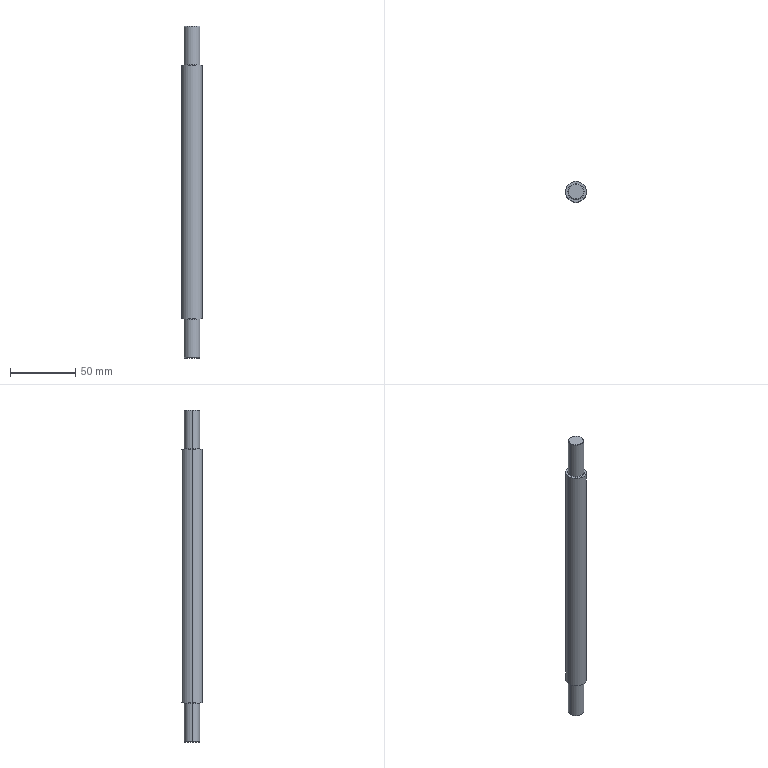Part | STEP file | 0230_002_MTSLW16-255-F30-V12-S30-Q12-BV15 | 1 solid | 18 faces | box 16 x 16 x 255 mm | volume 45988 mm3 | cylinder 6 | cone 4 | torus 4 | plane 4 | commonest cylinder face diameters 12 x4 16 x2
STEP:
#1=CARTESIAN_POINT('',(0.,0.,0.));
#2=DIRECTION('',(0.,0.,1.));
#3=DIRECTION('',(1.,0.,0.));
#4=AXIS2_PLACEMENT_3D('',#1,#2,#3);
#5=CARTESIAN_POINT('',(5.6,0.,30.));
#6=VERTEX_POINT('',#5);
#7=CARTESIAN_POINT('',(-5.6,0.,30.));
#8=VERTEX_POINT('',#7);
#9=CARTESIAN_POINT('',(0.,0.,30.));
#10=DIRECTION('',(0.,0.,1.));
#11=DIRECTION('',(1.,0.,0.));
#12=AXIS2_PLACEMENT_3D('',#9,#10,#11);
#13=CIRCLE('',#12,5.6);
#14=CARTESIAN_POINT('',(0.,0.,29.6));
#15=DIRECTION('',(0.,0.,-1.));
#16=DIRECTION('',(-1.,0.,0.));
#17=AXIS2_PLACEMENT_3D('',#14,#15,#16);
#18=CONICAL_SURFACE('',#17,6.,0.7854);
#19=CARTESIAN_POINT('',(3.142,-0.4));
#20=DIRECTION('',(-1.,0.));
#21=VECTOR('',#20,1.);
#22=LINE('',#19,#21);
#23=(GEOMETRIC_REPRESENTATION_CONTEXT(2)PARAMETRIC_REPRESENTATION_CONTEXT()REPRESENTATION_CONTEXT('',''));
#24=DEFINITIONAL_REPRESENTATION('',(#22),#23);
#25=PCURVE('',#18,#24);
#26=CARTESIAN_POINT('',(6.,0.,30.));
#27=DIRECTION('',(0.,0.,1.));
#28=DIRECTION('',(1.,0.,0.));
#29=AXIS2_PLACEMENT_3D('',#26,#27,#28);
#30=PLANE('',#29);
#31=CARTESIAN_POINT('',(-6.,0.));
#32=DIRECTION('',(1.,0.));
#33=AXIS2_PLACEMENT_2D('',#31,#32);
#34=CIRCLE('',#33,5.6);
#35=(GEOMETRIC_REPRESENTATION_CONTEXT(2)PARAMETRIC_REPRESENTATION_CONTEXT()REPRESENTATION_CONTEXT('',''));
#36=DEFINITIONAL_REPRESENTATION('',(#34),#35);
#37=PCURVE('',#30,#36);
#38=SURFACE_CURVE('',#13,(#25,#37),.PCURVE_S1.);
#39=EDGE_CURVE('',#6,#8,#38,.T.);
#40=ORIENTED_EDGE('',*,*,#39,.F.);
#41=CARTESIAN_POINT('',(6.,0.,29.6));
#42=VERTEX_POINT('',#41);
#43=CARTESIAN_POINT('',(6.,0.,29.6));
#44=DIRECTION('',(0.7071,0.,-0.7071));
#45=VECTOR('',#44,1.);
#46=LINE('',#43,#45);
#47=CARTESIAN_POINT('',(3.142,0.));
#48=DIRECTION('',(0.,1.));
#49=VECTOR('',#48,1.);
#50=LINE('',#47,#49);
#51=(GEOMETRIC_REPRESENTATION_CONTEXT(2)PARAMETRIC_REPRESENTATION_CONTEXT()REPRESENTATION_CONTEXT('',''));
#52=DEFINITIONAL_REPRESENTATION('',(#50),#51);
#53=PCURVE('',#18,#52);
#54=CARTESIAN_POINT('',(0.,0.,29.6));
#55=DIRECTION('',(0.,0.,-1.));
#56=DIRECTION('',(-1.,0.,0.));
#57=AXIS2_PLACEMENT_3D('',#54,#55,#56);
#58=CONICAL_SURFACE('',#57,6.,0.7854);
#59=CARTESIAN_POINT('',(3.142,0.));
#60=DIRECTION('',(0.,1.));
#61=VECTOR('',#60,1.);
#62=LINE('',#59,#61);
#63=(GEOMETRIC_REPRESENTATION_CONTEXT(2)PARAMETRIC_REPRESENTATION_CONTEXT()REPRESENTATION_CONTEXT('',''));
#64=DEFINITIONAL_REPRESENTATION('',(#62),#63);
#65=PCURVE('',#58,#64);
#66=SURFACE_CURVE('',#46,(#53,#65),.PCURVE_S1.);
#67=EDGE_CURVE('',#6,#42,#66,.T.);
#68=ORIENTED_EDGE('',*,*,#67,.T.);
#69=CARTESIAN_POINT('',(-6.,0.,29.6));
#70=VERTEX_POINT('',#69);
#71=CARTESIAN_POINT('',(0.,0.,29.6));
#72=DIRECTION('',(0.,0.,-1.));
#73=DIRECTION('',(1.,0.,0.));
#74=AXIS2_PLACEMENT_3D('',#71,#72,#73);
#75=CIRCLE('',#74,6.);
#76=CARTESIAN_POINT('',(-3.142,0.));
#77=DIRECTION('',(1.,0.));
#78=VECTOR('',#77,1.);
#79=LINE('',#76,#78);
#80=(GEOMETRIC_REPRESENTATION_CONTEXT(2)PARAMETRIC_REPRESENTATION_CONTEXT()REPRESENTATION_CONTEXT('',''));
#81=DEFINITIONAL_REPRESENTATION('',(#79),#80);
#82=PCURVE('',#18,#81);
#83=CARTESIAN_POINT('',(0.,0.,30.));
#84=DIRECTION('',(0.,0.,-1.));
#85=DIRECTION('',(-1.,0.,0.));
#86=AXIS2_PLACEMENT_3D('',#83,#84,#85);
#87=CYLINDRICAL_SURFACE('',#86,6.);
#88=CARTESIAN_POINT('',(-3.142,0.4));
#89=DIRECTION('',(1.,0.));
#90=VECTOR('',#89,1.);
#91=LINE('',#88,#90);
#92=(GEOMETRIC_REPRESENTATION_CONTEXT(2)PARAMETRIC_REPRESENTATION_CONTEXT()REPRESENTATION_CONTEXT('',''));
#93=DEFINITIONAL_REPRESENTATION('',(#91),#92);
#94=PCURVE('',#87,#93);
#95=SURFACE_CURVE('',#75,(#82,#94),.PCURVE_S1.);
#96=EDGE_CURVE('',#70,#42,#95,.T.);
#97=ORIENTED_EDGE('',*,*,#96,.F.);
#98=CARTESIAN_POINT('',(-6.,0.,29.6));
#99=DIRECTION('',(-0.7071,0.,-0.7071));
#100=VECTOR('',#99,1.);
#101=LINE('',#98,#100);
#102=CARTESIAN_POINT('',(0.,0.));
#103=DIRECTION('',(0.,1.));
#104=VECTOR('',#103,1.);
#105=LINE('',#102,#104);
#106=(GEOMETRIC_REPRESENTATION_CONTEXT(2)PARAMETRIC_REPRESENTATION_CONTEXT()REPRESENTATION_CONTEXT('',''));
#107=DEFINITIONAL_REPRESENTATION('',(#105),#106);
#108=PCURVE('',#18,#107);
#109=CARTESIAN_POINT('',(6.283,0.));
#110=DIRECTION('',(0.,1.));
#111=VECTOR('',#110,1.);
#112=LINE('',#109,#111);
#113=(GEOMETRIC_REPRESENTATION_CONTEXT(2)PARAMETRIC_REPRESENTATION_CONTEXT()REPRESENTATION_CONTEXT('',''));
#114=DEFINITIONAL_REPRESENTATION('',(#112),#113);
#115=PCURVE('',#58,#114);
#116=SURFACE_CURVE('',#101,(#108,#115),.PCURVE_S1.);
#117=EDGE_CURVE('',#8,#70,#116,.T.);
#118=ORIENTED_EDGE('',*,*,#117,.F.);
#119=EDGE_LOOP('',(#40,#68,#97,#118));
#120=FACE_BOUND('',#119,.T.);
#121=ADVANCED_FACE('',(#120),#18,.T.);
#122=CARTESIAN_POINT('',(-5.6,0.,-225.));
#123=VERTEX_POINT('',#122);
#124=CARTESIAN_POINT('',(5.6,0.,-225.));
#125=VERTEX_POINT('',#124);
#126=CARTESIAN_POINT('',(0.,0.,-225.));
#127=DIRECTION('',(0.,0.,-1.));
#128=DIRECTION('',(-1.,0.,0.));
#129=AXIS2_PLACEMENT_3D('',#126,#127,#128);
#130=CIRCLE('',#129,5.6);
#131=CARTESIAN_POINT('',(0.,0.,-225.));
#132=DIRECTION('',(0.,0.,1.));
#133=DIRECTION('',(1.,0.,0.));
#134=AXIS2_PLACEMENT_3D('',#131,#132,#133);
#135=CONICAL_SURFACE('',#134,5.6,0.7854);
#136=CARTESIAN_POINT('',(3.142,0.));
#137=DIRECTION('',(-1.,0.));
#138=VECTOR('',#137,1.);
#139=LINE('',#136,#138);
#140=(GEOMETRIC_REPRESENTATION_CONTEXT(2)PARAMETRIC_REPRESENTATION_CONTEXT()REPRESENTATION_CONTEXT('',''));
#141=DEFINITIONAL_REPRESENTATION('',(#139),#140);
#142=PCURVE('',#135,#141);
#143=CARTESIAN_POINT('',(0.,0.,-225.));
#144=DIRECTION('',(0.,0.,-1.));
#145=DIRECTION('',(-1.,0.,0.));
#146=AXIS2_PLACEMENT_3D('',#143,#144,#145);
#147=PLANE('',#146);
#148=CARTESIAN_POINT('',(0.,0.));
#149=DIRECTION('',(1.,0.));
#150=AXIS2_PLACEMENT_2D('',#148,#149);
#151=CIRCLE('',#150,5.6);
#152=(GEOMETRIC_REPRESENTATION_CONTEXT(2)PARAMETRIC_REPRESENTATION_CONTEXT()REPRESENTATION_CONTEXT('',''));
#153=DEFINITIONAL_REPRESENTATION('',(#151),#152);
#154=PCURVE('',#147,#153);
#155=SURFACE_CURVE('',#130,(#142,#154),.PCURVE_S1.);
#156=EDGE_CURVE('',#123,#125,#155,.T.);
#157=ORIENTED_EDGE('',*,*,#156,.F.);
#158=CARTESIAN_POINT('',(-6.,0.,-224.6));
#159=VERTEX_POINT('',#158);
#160=CARTESIAN_POINT('',(-5.6,0.,-225.));
#161=DIRECTION('',(-0.7071,0.,0.7071));
#162=VECTOR('',#161,1.);
#163=LINE('',#160,#162);
#164=CARTESIAN_POINT('',(3.142,0.));
#165=DIRECTION('',(0.,1.));
#166=VECTOR('',#165,1.);
#167=LINE('',#164,#166);
#168=(GEOMETRIC_REPRESENTATION_CONTEXT(2)PARAMETRIC_REPRESENTATION_CONTEXT()REPRESENTATION_CONTEXT('',''));
#169=DEFINITIONAL_REPRESENTATION('',(#167),#168);
#170=PCURVE('',#135,#169);
#171=CARTESIAN_POINT('',(0.,0.,-225.));
#172=DIRECTION('',(0.,0.,1.));
#173=DIRECTION('',(1.,0.,0.));
#174=AXIS2_PLACEMENT_3D('',#171,#172,#173);
#175=CONICAL_SURFACE('',#174,5.6,0.7854);
#176=CARTESIAN_POINT('',(3.142,0.));
#177=DIRECTION('',(0.,1.));
#178=VECTOR('',#177,1.);
#179=LINE('',#176,#178);
#180=(GEOMETRIC_REPRESENTATION_CONTEXT(2)PARAMETRIC_REPRESENTATION_CONTEXT()REPRESENTATION_CONTEXT('',''));
#181=DEFINITIONAL_REPRESENTATION('',(#179),#180);
#182=PCURVE('',#175,#181);
#183=SURFACE_CURVE('',#163,(#170,#182),.PCURVE_S1.);
#184=EDGE_CURVE('',#123,#159,#183,.T.);
#185=ORIENTED_EDGE('',*,*,#184,.T.);
#186=CARTESIAN_POINT('',(6.,0.,-224.6));
#187=VERTEX_POINT('',#186);
#188=CARTESIAN_POINT('',(0.,0.,-224.6));
#189=DIRECTION('',(0.,0.,1.));
#190=DIRECTION('',(-1.,0.,0.));
#191=AXIS2_PLACEMENT_3D('',#188,#189,#190);
#192=CIRCLE('',#191,6.);
#193=CARTESIAN_POINT('',(-3.142,0.4));
#194=DIRECTION('',(1.,0.));
#195=VECTOR('',#194,1.);
#196=LINE('',#193,#195);
#197=(GEOMETRIC_REPRESENTATION_CONTEXT(2)PARAMETRIC_REPRESENTATION_CONTEXT()REPRESENTATION_CONTEXT('',''));
#198=DEFINITIONAL_REPRESENTATION('',(#196),#197);
#199=PCURVE('',#135,#198);
#200=CARTESIAN_POINT('',(0.,0.,30.));
#201=DIRECTION('',(0.,0.,-1.));
#202=DIRECTION('',(-1.,0.,0.));
#203=AXIS2_PLACEMENT_3D('',#200,#201,#202);
#204=CYLINDRICAL_SURFACE('',#203,6.);
#205=CARTESIAN_POINT('',(6.283,254.6));
#206=DIRECTION('',(-1.,0.));
#207=VECTOR('',#206,1.);
#208=LINE('',#205,#207);
#209=(GEOMETRIC_REPRESENTATION_CONTEXT(2)PARAMETRIC_REPRESENTATION_CONTEXT()REPRESENTATION_CONTEXT('',''));
#210=DEFINITIONAL_REPRESENTATION('',(#208),#209);
#211=PCURVE('',#204,#210);
#212=SURFACE_CURVE('',#192,(#199,#211),.PCURVE_S1.);
#213=EDGE_CURVE('',#187,#159,#212,.T.);
#214=ORIENTED_EDGE('',*,*,#213,.F.);
#215=CARTESIAN_POINT('',(5.6,0.,-225.));
#216=DIRECTION('',(0.7071,0.,0.7071));
#217=VECTOR('',#216,1.);
#218=LINE('',#215,#217);
#219=CARTESIAN_POINT('',(0.,0.));
#220=DIRECTION('',(0.,1.));
#221=VECTOR('',#220,1.);
#222=LINE('',#219,#221);
#223=(GEOMETRIC_REPRESENTATION_CONTEXT(2)PARAMETRIC_REPRESENTATION_CONTEXT()REPRESENTATION_CONTEXT('',''));
#224=DEFINITIONAL_REPRESENTATION('',(#222),#223);
#225=PCURVE('',#135,#224);
#226=CARTESIAN_POINT('',(6.283,0.));
#227=DIRECTION('',(0.,1.));
#228=VECTOR('',#227,1.);
#229=LINE('',#226,#228);
#230=(GEOMETRIC_REPRESENTATION_CONTEXT(2)PARAMETRIC_REPRESENTATION_CONTEXT()REPRESENTATION_CONTEXT('',''));
#231=DEFINITIONAL_REPRESENTATION('',(#229),#230);
#232=PCURVE('',#175,#231);
#233=SURFACE_CURVE('',#218,(#225,#232),.PCURVE_S1.);
#234=EDGE_CURVE('',#125,#187,#233,.T.);
#235=ORIENTED_EDGE('',*,*,#234,.F.);
#236=EDGE_LOOP('',(#157,#185,#214,#235));
#237=FACE_BOUND('',#236,.T.);
#238=ADVANCED_FACE('',(#237),#135,.T.);
#239=CARTESIAN_POINT('',(6.,0.,0.3));
#240=VERTEX_POINT('',#239);
#241=CARTESIAN_POINT('',(6.3,0.,0.));
#242=VERTEX_POINT('',#241);
#243=CARTESIAN_POINT('',(6.3,0.,0.3));
#244=DIRECTION('',(0.,-1.,0.));
#245=DIRECTION('',(0.,0.,-1.));
#246=AXIS2_PLACEMENT_3D('',#243,#244,#245);
#247=CIRCLE('',#246,0.3);
#248=CARTESIAN_POINT('',(0.,0.,0.3));
#249=DIRECTION('',(0.,0.,1.));
#250=DIRECTION('',(1.,0.,0.));
#251=AXIS2_PLACEMENT_3D('',#248,#249,#250);
#252=TOROIDAL_SURFACE('',#251,6.3,0.3);
#253=CARTESIAN_POINT('',(6.283,-1.571));
#254=DIRECTION('',(0.,1.));
#255=VECTOR('',#254,1.);
#256=LINE('',#253,#255);
#257=(GEOMETRIC_REPRESENTATION_CONTEXT(2)PARAMETRIC_REPRESENTATION_CONTEXT()REPRESENTATION_CONTEXT('',''));
#258=DEFINITIONAL_REPRESENTATION('',(#256),#257);
#259=PCURVE('',#252,#258);
#260=CARTESIAN_POINT('',(0.,0.,0.3));
#261=DIRECTION('',(0.,0.,1.));
#262=DIRECTION('',(1.,0.,0.));
#263=AXIS2_PLACEMENT_3D('',#260,#261,#262);
#264=TOROIDAL_SURFACE('',#263,6.3,0.3);
#265=CARTESIAN_POINT('',(0.,-1.571));
#266=DIRECTION('',(0.,1.));
#267=VECTOR('',#266,1.);
#268=LINE('',#265,#267);
#269=(GEOMETRIC_REPRESENTATION_CONTEXT(2)PARAMETRIC_REPRESENTATION_CONTEXT()REPRESENTATION_CONTEXT('',''));
#270=DEFINITIONAL_REPRESENTATION('',(#268),#269);
#271=PCURVE('',#264,#270);
#272=SURFACE_CURVE('',#247,(#259,#271),.PCURVE_S1.);
#273=EDGE_CURVE('',#240,#242,#272,.T.);
#274=ORIENTED_EDGE('',*,*,#273,.T.);
#275=CARTESIAN_POINT('',(-6.3,0.,0.));
#276=VERTEX_POINT('',#275);
#277=CARTESIAN_POINT('',(0.,0.,0.));
#278=DIRECTION('',(0.,0.,-1.));
#279=DIRECTION('',(1.,0.,0.));
#280=AXIS2_PLACEMENT_3D('',#277,#278,#279);
#281=CIRCLE('',#280,6.3);
#282=CARTESIAN_POINT('',(6.283,4.712));
#283=DIRECTION('',(-1.,0.));
#284=VECTOR('',#283,1.);
#285=LINE('',#282,#284);
#286=(GEOMETRIC_REPRESENTATION_CONTEXT(2)PARAMETRIC_REPRESENTATION_CONTEXT()REPRESENTATION_CONTEXT('',''));
#287=DEFINITIONAL_REPRESENTATION('',(#285),#286);
#288=PCURVE('',#252,#287);
#289=CARTESIAN_POINT('',(8.,0.,0.));
#290=DIRECTION('',(0.,0.,1.));
#291=DIRECTION('',(1.,0.,0.));
#292=AXIS2_PLACEMENT_3D('',#289,#290,#291);
#293=PLANE('',#292);
#294=CARTESIAN_POINT('',(-1.7,0.));
#295=CARTESIAN_POINT('',(-1.7,-10.912));
#296=CARTESIAN_POINT('',(-11.15,-5.456));
#297=CARTESIAN_POINT('',(-20.6,0.));
#298=CARTESIAN_POINT('',(-11.15,5.456));
#299=CARTESIAN_POINT('',(-1.7,10.912));
#300=CARTESIAN_POINT('',(-1.7,0.));
#301=(BOUNDED_CURVE()B_SPLINE_CURVE(2,(#294,#295,#296,#297,#298,#299,#300),.UNSPECIFIED.,.T.,.F.)B_SPLINE_CURVE_WITH_KNOTS((1,2,2,2,2,1),(-2.094,0.,2.094,4.189,6.283,8.378),.UNSPECIFIED.)CURVE()GEOMETRIC_REPRESENTATION_ITEM()RATIONAL_B_SPLINE_CURVE((1.,0.5,1.,0.5,1.,0.5,1.))REPRESENTATION_ITEM(''));
#302=(GEOMETRIC_REPRESENTATION_CONTEXT(2)PARAMETRIC_REPRESENTATION_CONTEXT()REPRESENTATION_CONTEXT('',''));
#303=DEFINITIONAL_REPRESENTATION('',(#301),#302);
#304=PCURVE('',#293,#303);
#305=SURFACE_CURVE('',#281,(#288,#304),.PCURVE_S1.);
#306=EDGE_CURVE('',#242,#276,#305,.T.);
#307=ORIENTED_EDGE('',*,*,#306,.T.);
#308=CARTESIAN_POINT('',(-6.,0.,0.3));
#309=VERTEX_POINT('',#308);
#310=CARTESIAN_POINT('',(-6.3,0.,0.3));
#311=DIRECTION('',(0.,1.,0.));
#312=DIRECTION('',(-1.,0.,0.));
#313=AXIS2_PLACEMENT_3D('',#310,#311,#312);
#314=CIRCLE('',#313,0.3);
#315=CARTESIAN_POINT('',(3.142,0.));
#316=DIRECTION('',(0.,1.));
#317=VECTOR('',#316,1.);
#318=LINE('',#315,#317);
#319=(GEOMETRIC_REPRESENTATION_CONTEXT(2)PARAMETRIC_REPRESENTATION_CONTEXT()REPRESENTATION_CONTEXT('',''));
#320=DEFINITIONAL_REPRESENTATION('',(#318),#319);
#321=PCURVE('',#252,#320);
#322=CARTESIAN_POINT('',(3.142,0.));
#323=DIRECTION('',(0.,1.));
#324=VECTOR('',#323,1.);
#325=LINE('',#322,#324);
#326=(GEOMETRIC_REPRESENTATION_CONTEXT(2)PARAMETRIC_REPRESENTATION_CONTEXT()REPRESENTATION_CONTEXT('',''));
#327=DEFINITIONAL_REPRESENTATION('',(#325),#326);
#328=PCURVE('',#264,#327);
#329=SURFACE_CURVE('',#314,(#321,#328),.PCURVE_S1.);
#330=EDGE_CURVE('',#309,#276,#329,.T.);
#331=ORIENTED_EDGE('',*,*,#330,.F.);
#332=CARTESIAN_POINT('',(0.,0.,0.3));
#333=DIRECTION('',(0.,0.,1.));
#334=DIRECTION('',(1.,0.,0.));
#335=AXIS2_PLACEMENT_3D('',#332,#333,#334);
#336=CIRCLE('',#335,6.);
#337=CARTESIAN_POINT('',(0.,3.142));
#338=DIRECTION('',(1.,0.));
#339=VECTOR('',#338,1.);
#340=LINE('',#337,#339);
#341=(GEOMETRIC_REPRESENTATION_CONTEXT(2)PARAMETRIC_REPRESENTATION_CONTEXT()REPRESENTATION_CONTEXT('',''));
#342=DEFINITIONAL_REPRESENTATION('',(#340),#341);
#343=PCURVE('',#252,#342);
#344=CARTESIAN_POINT('',(0.,0.,30.));
#345=DIRECTION('',(0.,0.,-1.));
#346=DIRECTION('',(-1.,0.,0.));
#347=AXIS2_PLACEMENT_3D('',#344,#345,#346);
#348=CYLINDRICAL_SURFACE('',#347,6.);
#349=CARTESIAN_POINT('',(9.425,29.7));
#350=DIRECTION('',(-1.,0.));
#351=VECTOR('',#350,1.);
#352=LINE('',#349,#351);
#353=(GEOMETRIC_REPRESENTATION_CONTEXT(2)PARAMETRIC_REPRESENTATION_CONTEXT()REPRESENTATION_CONTEXT('',''));
#354=DEFINITIONAL_REPRESENTATION('',(#352),#353);
#355=PCURVE('',#348,#354);
#356=SURFACE_CURVE('',#336,(#343,#355),.PCURVE_S1.);
#357=EDGE_CURVE('',#309,#240,#356,.T.);
#358=ORIENTED_EDGE('',*,*,#357,.T.);
#359=EDGE_LOOP('',(#274,#307,#331,#358));
#360=FACE_BOUND('',#359,.F.);
#361=ADVANCED_FACE('',(#360),#252,.F.);
#362=CARTESIAN_POINT('',(-6.,0.,-195.3));
#363=VERTEX_POINT('',#362);
#364=CARTESIAN_POINT('',(-6.3,0.,-195.));
#365=VERTEX_POINT('',#364);
#366=CARTESIAN_POINT('',(-6.3,0.,-195.3));
#367=DIRECTION('',(0.,-1.,0.));
#368=DIRECTION('',(0.,0.,-1.));
#369=AXIS2_PLACEMENT_3D('',#366,#367,#368);
#370=CIRCLE('',#369,0.3);
#371=CARTESIAN_POINT('',(0.,0.,-195.3));
#372=DIRECTION('',(0.,0.,-1.));
#373=DIRECTION('',(-1.,0.,0.));
#374=AXIS2_PLACEMENT_3D('',#371,#372,#373);
#375=TOROIDAL_SURFACE('',#374,6.3,0.3);
#376=CARTESIAN_POINT('',(6.283,1.571));
#377=DIRECTION('',(0.,1.));
#378=VECTOR('',#377,1.);
#379=LINE('',#376,#378);
#380=(GEOMETRIC_REPRESENTATION_CONTEXT(2)PARAMETRIC_REPRESENTATION_CONTEXT()REPRESENTATION_CONTEXT('',''));
#381=DEFINITIONAL_REPRESENTATION('',(#379),#380);
#382=PCURVE('',#375,#381);
#383=CARTESIAN_POINT('',(0.,0.,-195.3));
#384=DIRECTION('',(0.,0.,-1.));
#385=DIRECTION('',(-1.,0.,0.));
#386=AXIS2_PLACEMENT_3D('',#383,#384,#385);
#387=TOROIDAL_SURFACE('',#386,6.3,0.3);
#388=CARTESIAN_POINT('',(0.,1.571));
#389=DIRECTION('',(0.,1.));
#390=VECTOR('',#389,1.);
#391=LINE('',#388,#390);
#392=(GEOMETRIC_REPRESENTATION_CONTEXT(2)PARAMETRIC_REPRESENTATION_CONTEXT()REPRESENTATION_CONTEXT('',''));
#393=DEFINITIONAL_REPRESENTATION('',(#391),#392);
#394=PCURVE('',#387,#393);
#395=SURFACE_CURVE('',#370,(#382,#394),.PCURVE_S1.);
#396=EDGE_CURVE('',#363,#365,#395,.T.);
#397=ORIENTED_EDGE('',*,*,#396,.T.);
#398=CARTESIAN_POINT('',(6.3,0.,-195.));
#399=VERTEX_POINT('',#398);
#400=CARTESIAN_POINT('',(0.,0.,-195.));
#401=DIRECTION('',(0.,0.,1.));
#402=DIRECTION('',(-1.,0.,0.));
#403=AXIS2_PLACEMENT_3D('',#400,#401,#402);
#404=CIRCLE('',#403,6.3);
#405=CARTESIAN_POINT('',(6.283,4.712));
#406=DIRECTION('',(-1.,0.));
#407=VECTOR('',#406,1.);
#408=LINE('',#405,#407);
#409=(GEOMETRIC_REPRESENTATION_CONTEXT(2)PARAMETRIC_REPRESENTATION_CONTEXT()REPRESENTATION_CONTEXT('',''));
#410=DEFINITIONAL_REPRESENTATION('',(#408),#409);
#411=PCURVE('',#375,#410);
#412=CARTESIAN_POINT('',(6.,0.,-195.));
#413=DIRECTION('',(0.,0.,-1.));
#414=DIRECTION('',(-1.,0.,0.));
#415=AXIS2_PLACEMENT_3D('',#412,#413,#414);
#416=PLANE('',#415);
#417=CARTESIAN_POINT('',(12.3,0.));
#418=CARTESIAN_POINT('',(12.3,-10.912));
#419=CARTESIAN_POINT('',(2.85,-5.456));
#420=CARTESIAN_POINT('',(-6.6,0.));
#421=CARTESIAN_POINT('',(2.85,5.456));
#422=CARTESIAN_POINT('',(12.3,10.912));
#423=CARTESIAN_POINT('',(12.3,0.));
#424=(BOUNDED_CURVE()B_SPLINE_CURVE(2,(#417,#418,#419,#420,#421,#422,#423),.UNSPECIFIED.,.T.,.F.)B_SPLINE_CURVE_WITH_KNOTS((1,2,2,2,2,1),(-2.094,0.,2.094,4.189,6.283,8.378),.UNSPECIFIED.)CURVE()GEOMETRIC_REPRESENTATION_ITEM()RATIONAL_B_SPLINE_CURVE((1.,0.5,1.,0.5,1.,0.5,1.))REPRESENTATION_ITEM(''));
#425=(GEOMETRIC_REPRESENTATION_CONTEXT(2)PARAMETRIC_REPRESENTATION_CONTEXT()REPRESENTATION_CONTEXT('',''));
#426=DEFINITIONAL_REPRESENTATION('',(#424),#425);
#427=PCURVE('',#416,#426);
#428=SURFACE_CURVE('',#404,(#411,#427),.PCURVE_S1.);
#429=EDGE_CURVE('',#365,#399,#428,.T.);
#430=ORIENTED_EDGE('',*,*,#429,.T.);
#431=CARTESIAN_POINT('',(6.,0.,-195.3));
#432=VERTEX_POINT('',#431);
#433=CARTESIAN_POINT('',(6.3,0.,-195.3));
#434=DIRECTION('',(0.,1.,0.));
#435=DIRECTION('',(-1.,0.,0.));
#436=AXIS2_PLACEMENT_3D('',#433,#434,#435);
#437=CIRCLE('',#436,0.3);
#438=CARTESIAN_POINT('',(3.142,3.142));
#439=DIRECTION('',(0.,1.));
#440=VECTOR('',#439,1.);
#441=LINE('',#438,#440);
#442=(GEOMETRIC_REPRESENTATION_CONTEXT(2)PARAMETRIC_REPRESENTATION_CONTEXT()REPRESENTATION_CONTEXT('',''));
#443=DEFINITIONAL_REPRESENTATION('',(#441),#442);
#444=PCURVE('',#375,#443);
#445=CARTESIAN_POINT('',(3.142,3.142));
#446=DIRECTION('',(0.,1.));
#447=VECTOR('',#446,1.);
#448=LINE('',#445,#447);
#449=(GEOMETRIC_REPRESENTATION_CONTEXT(2)PARAMETRIC_REPRESENTATION_CONTEXT()REPRESENTATION_CONTEXT('',''));
#450=DEFINITIONAL_REPRESENTATION('',(#448),#449);
#451=PCURVE('',#387,#450);
#452=SURFACE_CURVE('',#437,(#444,#451),.PCURVE_S1.);
#453=EDGE_CURVE('',#432,#399,#452,.T.);
#454=ORIENTED_EDGE('',*,*,#453,.F.);
#455=CARTESIAN_POINT('',(0.,0.,-195.3));
#456=DIRECTION('',(0.,0.,-1.));
#457=DIRECTION('',(-1.,0.,0.));
#458=AXIS2_PLACEMENT_3D('',#455,#456,#457);
#459=CIRCLE('',#458,6.);
#460=CARTESIAN_POINT('',(0.,3.142));
#461=DIRECTION('',(1.,0.));
#462=VECTOR('',#461,1.);
#463=LINE('',#460,#462);
#464=(GEOMETRIC_REPRESENTATION_CONTEXT(2)PARAMETRIC_REPRESENTATION_CONTEXT()REPRESENTATION_CONTEXT('',''));
#465=DEFINITIONAL_REPRESENTATION('',(#463),#464);
#466=PCURVE('',#375,#465);
#467=CARTESIAN_POINT('',(0.,0.,30.));
#468=DIRECTION('',(0.,0.,-1.));
#469=DIRECTION('',(-1.,0.,0.));
#470=AXIS2_PLACEMENT_3D('',#467,#468,#469);
#471=CYLINDRICAL_SURFACE('',#470,6.);
#472=CARTESIAN_POINT('',(0.,225.3));
#473=DIRECTION('',(1.,0.));
#474=VECTOR('',#473,1.);
#475=LINE('',#472,#474);
#476=(GEOMETRIC_REPRESENTATION_CONTEXT(2)PARAMETRIC_REPRESENTATION_CONTEXT()REPRESENTATION_CONTEXT('',''));
#477=DEFINITIONAL_REPRESENTATION('',(#475),#476);
#478=PCURVE('',#471,#477);
#479=SURFACE_CURVE('',#459,(#466,#478),.PCURVE_S1.);
#480=EDGE_CURVE('',#432,#363,#479,.T.);
#481=ORIENTED_EDGE('',*,*,#480,.T.);
#482=EDGE_LOOP('',(#397,#430,#454,#481));
#483=FACE_BOUND('',#482,.F.);
#484=ADVANCED_FACE('',(#483),#375,.F.);
#485=CARTESIAN_POINT('',(-8.,0.,0.));
#486=VERTEX_POINT('',#485);
#487=CARTESIAN_POINT('',(8.,0.,0.));
#488=VERTEX_POINT('',#487);
#489=CARTESIAN_POINT('',(0.,0.,0.));
#490=DIRECTION('',(0.,0.,-1.));
#491=DIRECTION('',(-1.,0.,0.));
#492=AXIS2_PLACEMENT_3D('',#489,#490,#491);
#493=CIRCLE('',#492,8.);
#494=CARTESIAN_POINT('',(0.,0.,30.));
#495=DIRECTION('',(0.,0.,-1.));
#496=DIRECTION('',(-1.,0.,0.));
#497=AXIS2_PLACEMENT_3D('',#494,#495,#496);
#498=CYLINDRICAL_SURFACE('',#497,8.);
#499=CARTESIAN_POINT('',(0.,30.));
#500=DIRECTION('',(1.,0.));
#501=VECTOR('',#500,1.);
#502=LINE('',#499,#501);
#503=(GEOMETRIC_REPRESENTATION_CONTEXT(2)PARAMETRIC_REPRESENTATION_CONTEXT()REPRESENTATION_CONTEXT('',''));
#504=DEFINITIONAL_REPRESENTATION('',(#502),#503);
#505=PCURVE('',#498,#504);
#506=CARTESIAN_POINT('',(-16.,0.));
#507=CARTESIAN_POINT('',(-16.,13.856));
#508=CARTESIAN_POINT('',(-4.,6.928));
#509=CARTESIAN_POINT('',(8.,0.));
#510=CARTESIAN_POINT('',(-4.,-6.928));
#511=CARTESIAN_POINT('',(-16.,-13.856));
#512=CARTESIAN_POINT('',(-16.,0.));
#513=(BOUNDED_CURVE()B_SPLINE_CURVE(2,(#506,#507,#508,#509,#510,#511,#512),.UNSPECIFIED.,.T.,.F.)B_SPLINE_CURVE_WITH_KNOTS((1,2,2,2,2,1),(-2.094,0.,2.094,4.189,6.283,8.378),.UNSPECIFIED.)CURVE()GEOMETRIC_REPRESENTATION_ITEM()RATIONAL_B_SPLINE_CURVE((1.,0.5,1.,0.5,1.,0.5,1.))REPRESENTATION_ITEM(''));
#514=(GEOMETRIC_REPRESENTATION_CONTEXT(2)PARAMETRIC_REPRESENTATION_CONTEXT()REPRESENTATION_CONTEXT('',''));
#515=DEFINITIONAL_REPRESENTATION('',(#513),#514);
#516=PCURVE('',#293,#515);
#517=SURFACE_CURVE('',#493,(#505,#516),.PCURVE_S1.);
#518=EDGE_CURVE('',#486,#488,#517,.T.);
#519=ORIENTED_EDGE('',*,*,#518,.T.);
#520=CARTESIAN_POINT('',(8.,0.,-195.));
#521=VERTEX_POINT('',#520);
#522=CARTESIAN_POINT('',(8.,0.,30.));
#523=DIRECTION('',(0.,0.,-1.));
#524=VECTOR('',#523,1.);
#525=LINE('',#522,#524);
#526=CARTESIAN_POINT('',(3.142,0.));
#527=DIRECTION('',(0.,1.));
#528=VECTOR('',#527,1.);
#529=LINE('',#526,#528);
#530=(GEOMETRIC_REPRESENTATION_CONTEXT(2)PARAMETRIC_REPRESENTATION_CONTEXT()REPRESENTATION_CONTEXT('',''));
#531=DEFINITIONAL_REPRESENTATION('',(#529),#530);
#532=PCURVE('',#498,#531);
#533=CARTESIAN_POINT('',(0.,0.,30.));
#534=DIRECTION('',(0.,0.,-1.));
#535=DIRECTION('',(-1.,0.,0.));
#536=AXIS2_PLACEMENT_3D('',#533,#534,#535);
#537=CYLINDRICAL_SURFACE('',#536,8.);
#538=CARTESIAN_POINT('',(3.142,0.));
#539=DIRECTION('',(0.,1.));
#540=VECTOR('',#539,1.);
#541=LINE('',#538,#540);
#542=(GEOMETRIC_REPRESENTATION_CONTEXT(2)PARAMETRIC_REPRESENTATION_CONTEXT()REPRESENTATION_CONTEXT('',''));
#543=DEFINITIONAL_REPRESENTATION('',(#541),#542);
#544=PCURVE('',#537,#543);
#545=SURFACE_CURVE('',#525,(#532,#544),.PCURVE_S1.);
#546=EDGE_CURVE('',#488,#521,#545,.T.);
#547=ORIENTED_EDGE('',*,*,#546,.T.);
#548=CARTESIAN_POINT('',(-8.,0.,-195.));
#549=VERTEX_POINT('',#548);
#550=CARTESIAN_POINT('',(0.,0.,-195.));
#551=DIRECTION('',(0.,0.,-1.));
#552=DIRECTION('',(-1.,0.,0.));
#553=AXIS2_PLACEMENT_3D('',#550,#551,#552);
#554=CIRCLE('',#553,8.);
#555=CARTESIAN_POINT('',(0.,225.));
#556=DIRECTION('',(1.,0.));
#557=VECTOR('',#556,1.);
#558=LINE('',#555,#557);
#559=(GEOMETRIC_REPRESENTATION_CONTEXT(2)PARAMETRIC_REPRESENTATION_CONTEXT()REPRESENTATION_CONTEXT('',''));
#560=DEFINITIONAL_REPRESENTATION('',(#558),#559);
#561=PCURVE('',#498,#560);
#562=CARTESIAN_POINT('',(6.,0.));
#563=DIRECTION('',(1.,0.));
#564=AXIS2_PLACEMENT_2D('',#562,#563);
#565=CIRCLE('',#564,8.);
#566=(GEOMETRIC_REPRESENTATION_CONTEXT(2)PARAMETRIC_REPRESENTATION_CONTEXT()REPRESENTATION_CONTEXT('',''));
#567=DEFINITIONAL_REPRESENTATION('',(#565),#566);
#568=PCURVE('',#416,#567);
#569=SURFACE_CURVE('',#554,(#561,#568),.PCURVE_S1.);
#570=EDGE_CURVE('',#549,#521,#569,.T.);
#571=ORIENTED_EDGE('',*,*,#570,.F.);
#572=CARTESIAN_POINT('',(-8.,0.,30.));
#573=DIRECTION('',(0.,0.,-1.));
#574=VECTOR('',#573,1.);
#575=LINE('',#572,#574);
#576=CARTESIAN_POINT('',(0.,0.));
#577=DIRECTION('',(0.,1.));
#578=VECTOR('',#577,1.);
#579=LINE('',#576,#578);
#580=(GEOMETRIC_REPRESENTATION_CONTEXT(2)PARAMETRIC_REPRESENTATION_CONTEXT()REPRESENTATION_CONTEXT('',''));
#581=DEFINITIONAL_REPRESENTATION('',(#579),#580);
#582=PCURVE('',#498,#581);
#583=CARTESIAN_POINT('',(6.283,0.));
#584=DIRECTION('',(0.,1.));
#585=VECTOR('',#584,1.);
#586=LINE('',#583,#585);
#587=(GEOMETRIC_REPRESENTATION_CONTEXT(2)PARAMETRIC_REPRESENTATION_CONTEXT()REPRESENTATION_CONTEXT('',''));
#588=DEFINITIONAL_REPRESENTATION('',(#586),#587);
#589=PCURVE('',#537,#588);
#590=SURFACE_CURVE('',#575,(#582,#589),.PCURVE_S1.);
#591=EDGE_CURVE('',#486,#549,#590,.T.);
#592=ORIENTED_EDGE('',*,*,#591,.F.);
#593=EDGE_LOOP('',(#519,#547,#571,#592));
#594=FACE_BOUND('',#593,.T.);
#595=ADVANCED_FACE('',(#594),#498,.T.);
#596=CARTESIAN_POINT('',(0.,0.,-195.3));
#597=DIRECTION('',(0.,0.,-1.));
#598=DIRECTION('',(-1.,0.,0.));
#599=AXIS2_PLACEMENT_3D('',#596,#597,#598);
#600=CIRCLE('',#599,6.);
#601=CARTESIAN_POINT('',(0.,225.3));
#602=DIRECTION('',(1.,0.));
#603=VECTOR('',#602,1.);
#604=LINE('',#601,#603);
#605=(GEOMETRIC_REPRESENTATION_CONTEXT(2)PARAMETRIC_REPRESENTATION_CONTEXT()REPRESENTATION_CONTEXT('',''));
#606=DEFINITIONAL_REPRESENTATION('',(#604),#605);
#607=PCURVE('',#204,#606);
#608=CARTESIAN_POINT('',(0.,3.142));
#609=DIRECTION('',(1.,0.));
#610=VECTOR('',#609,1.);
#611=LINE('',#608,#610);
#612=(GEOMETRIC_REPRESENTATION_CONTEXT(2)PARAMETRIC_REPRESENTATION_CONTEXT()REPRESENTATION_CONTEXT('',''));
#613=DEFINITIONAL_REPRESENTATION('',(#611),#612);
#614=PCURVE('',#387,#613);
#615=SURFACE_CURVE('',#600,(#607,#614),.PCURVE_S1.);
#616=EDGE_CURVE('',#363,#432,#615,.T.);
#617=ORIENTED_EDGE('',*,*,#616,.T.);
#618=CARTESIAN_POINT('',(6.,0.,30.));
#619=DIRECTION('',(0.,0.,-1.));
#620=VECTOR('',#619,1.);
#621=LINE('',#618,#620);
#622=CARTESIAN_POINT('',(3.142,0.));
#623=DIRECTION('',(0.,1.));
#624=VECTOR('',#623,1.);
#625=LINE('',#622,#624);
#626=(GEOMETRIC_REPRESENTATION_CONTEXT(2)PARAMETRIC_REPRESENTATION_CONTEXT()REPRESENTATION_CONTEXT('',''));
#627=DEFINITIONAL_REPRESENTATION('',(#625),#626);
#628=PCURVE('',#204,#627);
#629=CARTESIAN_POINT('',(3.142,0.));
#630=DIRECTION('',(0.,1.));
#631=VECTOR('',#630,1.);
#632=LINE('',#629,#631);
#633=(GEOMETRIC_REPRESENTATION_CONTEXT(2)PARAMETRIC_REPRESENTATION_CONTEXT()REPRESENTATION_CONTEXT('',''));
#634=DEFINITIONAL_REPRESENTATION('',(#632),#633);
#635=PCURVE('',#471,#634);
#636=SURFACE_CURVE('',#621,(#628,#635),.PCURVE_S1.);
#637=EDGE_CURVE('',#432,#187,#636,.T.);
#638=ORIENTED_EDGE('',*,*,#637,.T.);
#639=ORIENTED_EDGE('',*,*,#213,.T.);
#640=CARTESIAN_POINT('',(-6.,0.,30.));
#641=DIRECTION('',(0.,0.,-1.));
#642=VECTOR('',#641,1.);
#643=LINE('',#640,#642);
#644=CARTESIAN_POINT('',(0.,0.));
#645=DIRECTION('',(0.,1.));
#646=VECTOR('',#645,1.);
#647=LINE('',#644,#646);
#648=(GEOMETRIC_REPRESENTATION_CONTEXT(2)PARAMETRIC_REPRESENTATION_CONTEXT()REPRESENTATION_CONTEXT('',''));
#649=DEFINITIONAL_REPRESENTATION('',(#647),#648);
#650=PCURVE('',#204,#649);
#651=CARTESIAN_POINT('',(6.283,0.));
#652=DIRECTION('',(0.,1.));
#653=VECTOR('',#652,1.);
#654=LINE('',#651,#653);
#655=(GEOMETRIC_REPRESENTATION_CONTEXT(2)PARAMETRIC_REPRESENTATION_CONTEXT()REPRESENTATION_CONTEXT('',''));
#656=DEFINITIONAL_REPRESENTATION('',(#654),#655);
#657=PCURVE('',#471,#656);
#658=SURFACE_CURVE('',#643,(#650,#657),.PCURVE_S1.);
#659=EDGE_CURVE('',#363,#159,#658,.T.);
#660=ORIENTED_EDGE('',*,*,#659,.F.);
#661=EDGE_LOOP('',(#617,#638,#639,#660));
#662=FACE_BOUND('',#661,.T.);
#663=ADVANCED_FACE('',(#662),#204,.T.);
#664=ORIENTED_EDGE('',*,*,#96,.T.);
#665=CARTESIAN_POINT('',(6.,0.,30.));
#666=DIRECTION('',(0.,0.,-1.));
#667=VECTOR('',#666,1.);
#668=LINE('',#665,#667);
#669=CARTESIAN_POINT('',(3.142,0.));
#670=DIRECTION('',(0.,1.));
#671=VECTOR('',#670,1.);
#672=LINE('',#669,#671);
#673=(GEOMETRIC_REPRESENTATION_CONTEXT(2)PARAMETRIC_REPRESENTATION_CONTEXT()REPRESENTATION_CONTEXT('',''));
#674=DEFINITIONAL_REPRESENTATION('',(#672),#673);
#675=PCURVE('',#87,#674);
#676=CARTESIAN_POINT('',(3.142,0.));
#677=DIRECTION('',(0.,1.));
#678=VECTOR('',#677,1.);
#679=LINE('',#676,#678);
#680=(GEOMETRIC_REPRESENTATION_CONTEXT(2)PARAMETRIC_REPRESENTATION_CONTEXT()REPRESENTATION_CONTEXT('',''));
#681=DEFINITIONAL_REPRESENTATION('',(#679),#680);
#682=PCURVE('',#348,#681);
#683=SURFACE_CURVE('',#668,(#675,#682),.PCURVE_S1.);
#684=EDGE_CURVE('',#42,#240,#683,.T.);
#685=ORIENTED_EDGE('',*,*,#684,.T.);
#686=CARTESIAN_POINT('',(0.,0.,0.3));
#687=DIRECTION('',(0.,0.,1.));
#688=DIRECTION('',(1.,0.,0.));
#689=AXIS2_PLACEMENT_3D('',#686,#687,#688);
#690=CIRCLE('',#689,6.);
#691=CARTESIAN_POINT('',(3.142,29.7));
#692=DIRECTION('',(-1.,0.));
#693=VECTOR('',#692,1.);
#694=LINE('',#691,#693);
#695=(GEOMETRIC_REPRESENTATION_CONTEXT(2)PARAMETRIC_REPRESENTATION_CONTEXT()REPRESENTATION_CONTEXT('',''));
#696=DEFINITIONAL_REPRESENTATION('',(#694),#695);
#697=PCURVE('',#87,#696);
#698=CARTESIAN_POINT('',(0.,3.142));
#699=DIRECTION('',(1.,0.));
#700=VECTOR('',#699,1.);
#701=LINE('',#698,#700);
#702=(GEOMETRIC_REPRESENTATION_CONTEXT(2)PARAMETRIC_REPRESENTATION_CONTEXT()REPRESENTATION_CONTEXT('',''));
#703=DEFINITIONAL_REPRESENTATION('',(#701),#702);
#704=PCURVE('',#264,#703);
#705=SURFACE_CURVE('',#690,(#697,#704),.PCURVE_S1.);
#706=EDGE_CURVE('',#240,#309,#705,.T.);
#707=ORIENTED_EDGE('',*,*,#706,.T.);
#708=CARTESIAN_POINT('',(-6.,0.,30.));
#709=DIRECTION('',(0.,0.,-1.));
#710=VECTOR('',#709,1.);
#711=LINE('',#708,#710);
#712=CARTESIAN_POINT('',(0.,0.));
#713=DIRECTION('',(0.,1.));
#714=VECTOR('',#713,1.);
#715=LINE('',#712,#714);
#716=(GEOMETRIC_REPRESENTATION_CONTEXT(2)PARAMETRIC_REPRESENTATION_CONTEXT()REPRESENTATION_CONTEXT('',''));
#717=DEFINITIONAL_REPRESENTATION('',(#715),#716);
#718=PCURVE('',#87,#717);
#719=CARTESIAN_POINT('',(6.283,0.));
#720=DIRECTION('',(0.,1.));
#721=VECTOR('',#720,1.);
#722=LINE('',#719,#721);
#723=(GEOMETRIC_REPRESENTATION_CONTEXT(2)PARAMETRIC_REPRESENTATION_CONTEXT()REPRESENTATION_CONTEXT('',''));
#724=DEFINITIONAL_REPRESENTATION('',(#722),#723);
#725=PCURVE('',#348,#724);
#726=SURFACE_CURVE('',#711,(#718,#725),.PCURVE_S1.);
#727=EDGE_CURVE('',#70,#309,#726,.T.);
#728=ORIENTED_EDGE('',*,*,#727,.F.);
#729=EDGE_LOOP('',(#664,#685,#707,#728));
#730=FACE_BOUND('',#729,.T.);
#731=ADVANCED_FACE('',(#730),#87,.T.);
#732=ORIENTED_EDGE('',*,*,#684,.F.);
#733=CARTESIAN_POINT('',(0.,0.,29.6));
#734=DIRECTION('',(0.,0.,-1.));
#735=DIRECTION('',(1.,0.,0.));
#736=AXIS2_PLACEMENT_3D('',#733,#734,#735);
#737=CIRCLE('',#736,6.);
#738=CARTESIAN_POINT('',(3.142,0.4));
#739=DIRECTION('',(1.,0.));
#740=VECTOR('',#739,1.);
#741=LINE('',#738,#740);
#742=(GEOMETRIC_REPRESENTATION_CONTEXT(2)PARAMETRIC_REPRESENTATION_CONTEXT()REPRESENTATION_CONTEXT('',''));
#743=DEFINITIONAL_REPRESENTATION('',(#741),#742);
#744=PCURVE('',#348,#743);
#745=CARTESIAN_POINT('',(3.142,0.));
#746=DIRECTION('',(1.,0.));
#747=VECTOR('',#746,1.);
#748=LINE('',#745,#747);
#749=(GEOMETRIC_REPRESENTATION_CONTEXT(2)PARAMETRIC_REPRESENTATION_CONTEXT()REPRESENTATION_CONTEXT('',''));
#750=DEFINITIONAL_REPRESENTATION('',(#748),#749);
#751=PCURVE('',#58,#750);
#752=SURFACE_CURVE('',#737,(#744,#751),.PCURVE_S1.);
#753=EDGE_CURVE('',#42,#70,#752,.T.);
#754=ORIENTED_EDGE('',*,*,#753,.T.);
#755=ORIENTED_EDGE('',*,*,#727,.T.);
#756=ORIENTED_EDGE('',*,*,#357,.T.);
#757=EDGE_LOOP('',(#732,#754,#755,#756));
#758=FACE_BOUND('',#757,.T.);
#759=ADVANCED_FACE('',(#758),#348,.T.);
#760=CARTESIAN_POINT('',(0.,0.,30.));
#761=DIRECTION('',(0.,0.,1.));
#762=DIRECTION('',(1.,0.,0.));
#763=AXIS2_PLACEMENT_3D('',#760,#761,#762);
#764=CIRCLE('',#763,5.6);
#765=CARTESIAN_POINT('',(-6.,0.));
#766=DIRECTION('',(1.,0.));
#767=AXIS2_PLACEMENT_2D('',#765,#766);
#768=CIRCLE('',#767,5.6);
#769=(GEOMETRIC_REPRESENTATION_CONTEXT(2)PARAMETRIC_REPRESENTATION_CONTEXT()REPRESENTATION_CONTEXT('',''));
#770=DEFINITIONAL_REPRESENTATION('',(#768),#769);
#771=PCURVE('',#30,#770);
#772=CARTESIAN_POINT('',(9.425,-0.4));
#773=DIRECTION('',(-1.,0.));
#774=VECTOR('',#773,1.);
#775=LINE('',#772,#774);
#776=(GEOMETRIC_REPRESENTATION_CONTEXT(2)PARAMETRIC_REPRESENTATION_CONTEXT()REPRESENTATION_CONTEXT('',''));
#777=DEFINITIONAL_REPRESENTATION('',(#775),#776);
#778=PCURVE('',#58,#777);
#779=SURFACE_CURVE('',#764,(#771,#778),.PCURVE_S1.);
#780=EDGE_CURVE('',#8,#6,#779,.T.);
#781=ORIENTED_EDGE('',*,*,#780,.T.);
#782=ORIENTED_EDGE('',*,*,#39,.T.);
#783=EDGE_LOOP('',(#781,#782));
#784=FACE_BOUND('',#783,.T.);
#785=ADVANCED_FACE('',(#784),#30,.T.);
#786=CARTESIAN_POINT('',(0.,0.,-225.));
#787=DIRECTION('',(0.,0.,-1.));
#788=DIRECTION('',(-1.,0.,0.));
#789=AXIS2_PLACEMENT_3D('',#786,#787,#788);
#790=CIRCLE('',#789,5.6);
#791=CARTESIAN_POINT('',(0.,0.));
#792=DIRECTION('',(1.,0.));
#793=AXIS2_PLACEMENT_2D('',#791,#792);
#794=CIRCLE('',#793,5.6);
#795=(GEOMETRIC_REPRESENTATION_CONTEXT(2)PARAMETRIC_REPRESENTATION_CONTEXT()REPRESENTATION_CONTEXT('',''));
#796=DEFINITIONAL_REPRESENTATION('',(#794),#795);
#797=PCURVE('',#147,#796);
#798=CARTESIAN_POINT('',(9.425,0.));
#799=DIRECTION('',(-1.,0.));
#800=VECTOR('',#799,1.);
#801=LINE('',#798,#800);
#802=(GEOMETRIC_REPRESENTATION_CONTEXT(2)PARAMETRIC_REPRESENTATION_CONTEXT()REPRESENTATION_CONTEXT('',''));
#803=DEFINITIONAL_REPRESENTATION('',(#801),#802);
#804=PCURVE('',#175,#803);
#805=SURFACE_CURVE('',#790,(#797,#804),.PCURVE_S1.);
#806=EDGE_CURVE('',#125,#123,#805,.T.);
#807=ORIENTED_EDGE('',*,*,#806,.T.);
#808=ORIENTED_EDGE('',*,*,#156,.T.);
#809=EDGE_LOOP('',(#807,#808));
#810=FACE_BOUND('',#809,.T.);
#811=ADVANCED_FACE('',(#810),#147,.T.);
#812=ORIENTED_EDGE('',*,*,#637,.F.);
#813=ORIENTED_EDGE('',*,*,#480,.T.);
#814=ORIENTED_EDGE('',*,*,#659,.T.);
#815=CARTESIAN_POINT('',(0.,0.,-224.6));
#816=DIRECTION('',(0.,0.,1.));
#817=DIRECTION('',(-1.,0.,0.));
#818=AXIS2_PLACEMENT_3D('',#815,#816,#817);
#819=CIRCLE('',#818,6.);
#820=CARTESIAN_POINT('',(6.283,254.6));
#821=DIRECTION('',(-1.,0.));
#822=VECTOR('',#821,1.);
#823=LINE('',#820,#822);
#824=(GEOMETRIC_REPRESENTATION_CONTEXT(2)PARAMETRIC_REPRESENTATION_CONTEXT()REPRESENTATION_CONTEXT('',''));
#825=DEFINITIONAL_REPRESENTATION('',(#823),#824);
#826=PCURVE('',#471,#825);
#827=CARTESIAN_POINT('',(3.142,0.4));
#828=DIRECTION('',(1.,0.));
#829=VECTOR('',#828,1.);
#830=LINE('',#827,#829);
#831=(GEOMETRIC_REPRESENTATION_CONTEXT(2)PARAMETRIC_REPRESENTATION_CONTEXT()REPRESENTATION_CONTEXT('',''));
#832=DEFINITIONAL_REPRESENTATION('',(#830),#831);
#833=PCURVE('',#175,#832);
#834=SURFACE_CURVE('',#819,(#826,#833),.PCURVE_S1.);
#835=EDGE_CURVE('',#159,#187,#834,.T.);
#836=ORIENTED_EDGE('',*,*,#835,.T.);
#837=EDGE_LOOP('',(#812,#813,#814,#836));
#838=FACE_BOUND('',#837,.T.);
#839=ADVANCED_FACE('',(#838),#471,.T.);
#840=ORIENTED_EDGE('',*,*,#429,.T.);
#841=CARTESIAN_POINT('',(0.,0.,-195.));
#842=DIRECTION('',(0.,0.,1.));
#843=DIRECTION('',(-1.,0.,0.));
#844=AXIS2_PLACEMENT_3D('',#841,#842,#843);
#845=CIRCLE('',#844,6.3);
#846=CARTESIAN_POINT('',(12.3,0.));
#847=CARTESIAN_POINT('',(12.3,-10.912));
#848=CARTESIAN_POINT('',(2.85,-5.456));
#849=CARTESIAN_POINT('',(-6.6,0.));
#850=CARTESIAN_POINT('',(2.85,5.456));
#851=CARTESIAN_POINT('',(12.3,10.912));
#852=CARTESIAN_POINT('',(12.3,0.));
#853=(BOUNDED_CURVE()B_SPLINE_CURVE(2,(#846,#847,#848,#849,#850,#851,#852),.UNSPECIFIED.,.T.,.F.)B_SPLINE_CURVE_WITH_KNOTS((1,2,2,2,2,1),(-2.094,0.,2.094,4.189,6.283,8.378),.UNSPECIFIED.)CURVE()GEOMETRIC_REPRESENTATION_ITEM()RATIONAL_B_SPLINE_CURVE((1.,0.5,1.,0.5,1.,0.5,1.))REPRESENTATION_ITEM(''));
#854=(GEOMETRIC_REPRESENTATION_CONTEXT(2)PARAMETRIC_REPRESENTATION_CONTEXT()REPRESENTATION_CONTEXT('',''));
#855=DEFINITIONAL_REPRESENTATION('',(#853),#854);
#856=PCURVE('',#416,#855);
#857=CARTESIAN_POINT('',(6.283,4.712));
#858=DIRECTION('',(-1.,0.));
#859=VECTOR('',#858,1.);
#860=LINE('',#857,#859);
#861=(GEOMETRIC_REPRESENTATION_CONTEXT(2)PARAMETRIC_REPRESENTATION_CONTEXT()REPRESENTATION_CONTEXT('',''));
#862=DEFINITIONAL_REPRESENTATION('',(#860),#861);
#863=PCURVE('',#387,#862);
#864=SURFACE_CURVE('',#845,(#856,#863),.PCURVE_S1.);
#865=EDGE_CURVE('',#399,#365,#864,.T.);
#866=ORIENTED_EDGE('',*,*,#865,.T.);
#867=EDGE_LOOP('',(#840,#866));
#868=FACE_BOUND('',#867,.T.);
#869=ORIENTED_EDGE('',*,*,#570,.T.);
#870=CARTESIAN_POINT('',(0.,0.,-195.));
#871=DIRECTION('',(0.,0.,-1.));
#872=DIRECTION('',(-1.,0.,0.));
#873=AXIS2_PLACEMENT_3D('',#870,#871,#872);
#874=CIRCLE('',#873,8.);
#875=CARTESIAN_POINT('',(6.,0.));
#876=DIRECTION('',(1.,0.));
#877=AXIS2_PLACEMENT_2D('',#875,#876);
#878=CIRCLE('',#877,8.);
#879=(GEOMETRIC_REPRESENTATION_CONTEXT(2)PARAMETRIC_REPRESENTATION_CONTEXT()REPRESENTATION_CONTEXT('',''));
#880=DEFINITIONAL_REPRESENTATION('',(#878),#879);
#881=PCURVE('',#416,#880);
#882=CARTESIAN_POINT('',(0.,225.));
#883=DIRECTION('',(1.,0.));
#884=VECTOR('',#883,1.);
#885=LINE('',#882,#884);
#886=(GEOMETRIC_REPRESENTATION_CONTEXT(2)PARAMETRIC_REPRESENTATION_CONTEXT()REPRESENTATION_CONTEXT('',''));
#887=DEFINITIONAL_REPRESENTATION('',(#885),#886);
#888=PCURVE('',#537,#887);
#889=SURFACE_CURVE('',#874,(#881,#888),.PCURVE_S1.);
#890=EDGE_CURVE('',#521,#549,#889,.T.);
#891=ORIENTED_EDGE('',*,*,#890,.T.);
#892=EDGE_LOOP('',(#869,#891));
#893=FACE_BOUND('',#892,.T.);
#894=ADVANCED_FACE('',(#868,#893),#416,.T.);
#895=ORIENTED_EDGE('',*,*,#546,.F.);
#896=CARTESIAN_POINT('',(0.,0.,0.));
#897=DIRECTION('',(0.,0.,-1.));
#898=DIRECTION('',(-1.,0.,0.));
#899=AXIS2_PLACEMENT_3D('',#896,#897,#898);
#900=CIRCLE('',#899,8.);
#901=CARTESIAN_POINT('',(0.,30.));
#902=DIRECTION('',(1.,0.));
#903=VECTOR('',#902,1.);
#904=LINE('',#901,#903);
#905=(GEOMETRIC_REPRESENTATION_CONTEXT(2)PARAMETRIC_REPRESENTATION_CONTEXT()REPRESENTATION_CONTEXT('',''));
#906=DEFINITIONAL_REPRESENTATION('',(#904),#905);
#907=PCURVE('',#537,#906);
#908=CARTESIAN_POINT('',(-16.,0.));
#909=CARTESIAN_POINT('',(-16.,13.856));
#910=CARTESIAN_POINT('',(-4.,6.928));
#911=CARTESIAN_POINT('',(8.,0.));
#912=CARTESIAN_POINT('',(-4.,-6.928));
#913=CARTESIAN_POINT('',(-16.,-13.856));
#914=CARTESIAN_POINT('',(-16.,0.));
#915=(BOUNDED_CURVE()B_SPLINE_CURVE(2,(#908,#909,#910,#911,#912,#913,#914),.UNSPECIFIED.,.T.,.F.)B_SPLINE_CURVE_WITH_KNOTS((1,2,2,2,2,1),(-2.094,0.,2.094,4.189,6.283,8.378),.UNSPECIFIED.)CURVE()GEOMETRIC_REPRESENTATION_ITEM()RATIONAL_B_SPLINE_CURVE((1.,0.5,1.,0.5,1.,0.5,1.))REPRESENTATION_ITEM(''));
#916=(GEOMETRIC_REPRESENTATION_CONTEXT(2)PARAMETRIC_REPRESENTATION_CONTEXT()REPRESENTATION_CONTEXT('',''));
#917=DEFINITIONAL_REPRESENTATION('',(#915),#916);
#918=PCURVE('',#293,#917);
#919=SURFACE_CURVE('',#900,(#907,#918),.PCURVE_S1.);
#920=EDGE_CURVE('',#488,#486,#919,.T.);
#921=ORIENTED_EDGE('',*,*,#920,.T.);
#922=ORIENTED_EDGE('',*,*,#591,.T.);
#923=ORIENTED_EDGE('',*,*,#890,.F.);
#924=EDGE_LOOP('',(#895,#921,#922,#923));
#925=FACE_BOUND('',#924,.T.);
#926=ADVANCED_FACE('',(#925),#537,.T.);
#927=ORIENTED_EDGE('',*,*,#306,.T.);
#928=CARTESIAN_POINT('',(0.,0.,0.));
#929=DIRECTION('',(0.,0.,-1.));
#930=DIRECTION('',(1.,0.,0.));
#931=AXIS2_PLACEMENT_3D('',#928,#929,#930);
#932=CIRCLE('',#931,6.3);
#933=CARTESIAN_POINT('',(-1.7,0.));
#934=CARTESIAN_POINT('',(-1.7,-10.912));
#935=CARTESIAN_POINT('',(-11.15,-5.456));
#936=CARTESIAN_POINT('',(-20.6,0.));
#937=CARTESIAN_POINT('',(-11.15,5.456));
#938=CARTESIAN_POINT('',(-1.7,10.912));
#939=CARTESIAN_POINT('',(-1.7,0.));
#940=(BOUNDED_CURVE()B_SPLINE_CURVE(2,(#933,#934,#935,#936,#937,#938,#939),.UNSPECIFIED.,.T.,.F.)B_SPLINE_CURVE_WITH_KNOTS((1,2,2,2,2,1),(-2.094,0.,2.094,4.189,6.283,8.378),.UNSPECIFIED.)CURVE()GEOMETRIC_REPRESENTATION_ITEM()RATIONAL_B_SPLINE_CURVE((1.,0.5,1.,0.5,1.,0.5,1.))REPRESENTATION_ITEM(''));
#941=(GEOMETRIC_REPRESENTATION_CONTEXT(2)PARAMETRIC_REPRESENTATION_CONTEXT()REPRESENTATION_CONTEXT('',''));
#942=DEFINITIONAL_REPRESENTATION('',(#940),#941);
#943=PCURVE('',#293,#942);
#944=CARTESIAN_POINT('',(6.283,4.712));
#945=DIRECTION('',(-1.,0.));
#946=VECTOR('',#945,1.);
#947=LINE('',#944,#946);
#948=(GEOMETRIC_REPRESENTATION_CONTEXT(2)PARAMETRIC_REPRESENTATION_CONTEXT()REPRESENTATION_CONTEXT('',''));
#949=DEFINITIONAL_REPRESENTATION('',(#947),#948);
#950=PCURVE('',#264,#949);
#951=SURFACE_CURVE('',#932,(#943,#950),.PCURVE_S1.);
#952=EDGE_CURVE('',#276,#242,#951,.T.);
#953=ORIENTED_EDGE('',*,*,#952,.T.);
#954=EDGE_LOOP('',(#927,#953));
#955=FACE_BOUND('',#954,.T.);
#956=ORIENTED_EDGE('',*,*,#518,.F.);
#957=ORIENTED_EDGE('',*,*,#920,.F.);
#958=EDGE_LOOP('',(#956,#957));
#959=FACE_BOUND('',#958,.T.);
#960=ADVANCED_FACE('',(#955,#959),#293,.T.);
#961=ORIENTED_EDGE('',*,*,#865,.T.);
#962=ORIENTED_EDGE('',*,*,#396,.F.);
#963=ORIENTED_EDGE('',*,*,#616,.T.);
#964=ORIENTED_EDGE('',*,*,#453,.T.);
#965=EDGE_LOOP('',(#961,#962,#963,#964));
#966=FACE_BOUND('',#965,.F.);
#967=ADVANCED_FACE('',(#966),#387,.F.);
#968=ORIENTED_EDGE('',*,*,#952,.T.);
#969=ORIENTED_EDGE('',*,*,#273,.F.);
#970=ORIENTED_EDGE('',*,*,#706,.T.);
#971=ORIENTED_EDGE('',*,*,#330,.T.);
#972=EDGE_LOOP('',(#968,#969,#970,#971));
#973=FACE_BOUND('',#972,.F.);
#974=ADVANCED_FACE('',(#973),#264,.F.);
#975=ORIENTED_EDGE('',*,*,#184,.F.);
#976=ORIENTED_EDGE('',*,*,#806,.F.);
#977=ORIENTED_EDGE('',*,*,#234,.T.);
#978=ORIENTED_EDGE('',*,*,#835,.F.);
#979=EDGE_LOOP('',(#975,#976,#977,#978));
#980=FACE_BOUND('',#979,.T.);
#981=ADVANCED_FACE('',(#980),#175,.T.);
#982=ORIENTED_EDGE('',*,*,#67,.F.);
#983=ORIENTED_EDGE('',*,*,#780,.F.);
#984=ORIENTED_EDGE('',*,*,#117,.T.);
#985=ORIENTED_EDGE('',*,*,#753,.F.);
#986=EDGE_LOOP('',(#982,#983,#984,#985));
#987=FACE_BOUND('',#986,.T.);
#988=ADVANCED_FACE('',(#987),#58,.T.);
#989=CLOSED_SHELL('',(#121,#238,#361,#484,#595,#663,#731,#759,#785,#811,#839,#894,#926,#960,#967,#974,#981,#988));
#990=MANIFOLD_SOLID_BREP('',#989);
#991=(LENGTH_UNIT()NAMED_UNIT(*)SI_UNIT(.MILLI.,.METRE.));
#992=UNCERTAINTY_MEASURE_WITH_UNIT(LENGTH_MEASURE(0.0000001),#991,'','');
#993=(NAMED_UNIT(*)PLANE_ANGLE_UNIT()SI_UNIT($,.RADIAN.));
#994=(NAMED_UNIT(*)SI_UNIT($,.STERADIAN.)SOLID_ANGLE_UNIT());
#995=(GEOMETRIC_REPRESENTATION_CONTEXT(3)GLOBAL_UNCERTAINTY_ASSIGNED_CONTEXT((#992))GLOBAL_UNIT_ASSIGNED_CONTEXT((#991,#993,#994))REPRESENTATION_CONTEXT('',''));
#996=ADVANCED_BREP_SHAPE_REPRESENTATION('',(#4,#990),#995);